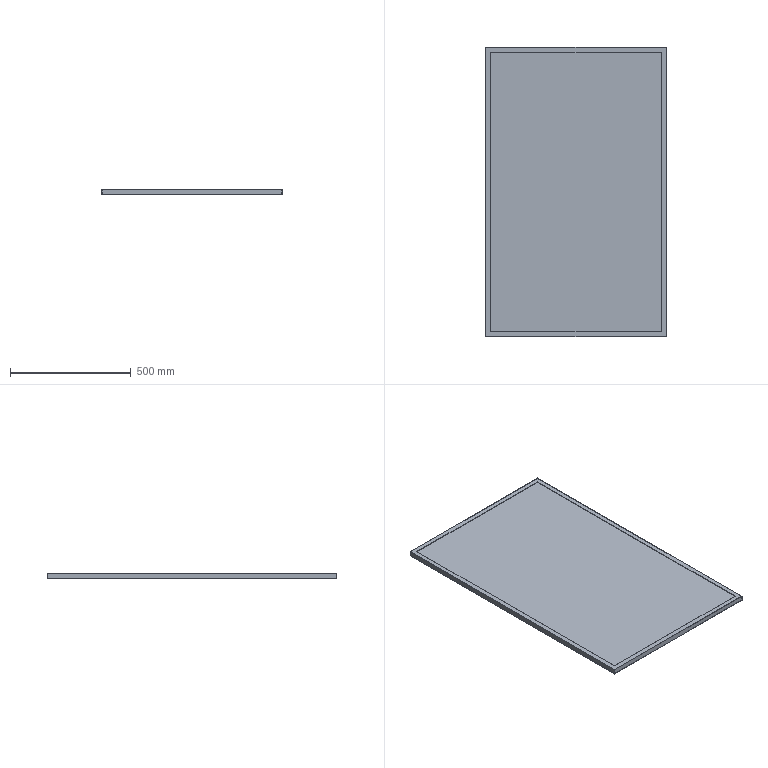Part | SolidWorks | features Extrusion 1, ICE 1, Shell 1 | 1 solid | 16 faces | box 745 x 1196 x 22 mm | volume 2073584 mm3 | plane 16
STEP:
#1=CARTESIAN_POINT('',(0.,1196.,22.));
#2=VERTEX_POINT('',#1);
#3=CARTESIAN_POINT('',(0.,0.,22.));
#4=VERTEX_POINT('',#3);
#5=CARTESIAN_POINT('',(0.,0.,22.));
#6=DIRECTION('',(0.,-1.,0.));
#7=VECTOR('',#6,1000.);
#8=LINE('',#5,#7);
#9=EDGE_CURVE('',#2,#4,#8,.T.);
#10=ORIENTED_EDGE('',*,*,#9,.T.);
#11=CARTESIAN_POINT('',(745.,0.,22.));
#12=VERTEX_POINT('',#11);
#13=CARTESIAN_POINT('',(0.,0.,22.));
#14=DIRECTION('',(1.,0.,0.));
#15=VECTOR('',#14,1000.);
#16=LINE('',#13,#15);
#17=EDGE_CURVE('',#4,#12,#16,.T.);
#18=ORIENTED_EDGE('',*,*,#17,.T.);
#19=CARTESIAN_POINT('',(745.,1196.,22.));
#20=VERTEX_POINT('',#19);
#21=CARTESIAN_POINT('',(745.,0.,22.));
#22=DIRECTION('',(0.,1.,0.));
#23=VECTOR('',#22,1000.);
#24=LINE('',#21,#23);
#25=EDGE_CURVE('',#12,#20,#24,.T.);
#26=ORIENTED_EDGE('',*,*,#25,.T.);
#27=CARTESIAN_POINT('',(0.,1196.,22.));
#28=DIRECTION('',(-1.,0.,0.));
#29=VECTOR('',#28,1000.);
#30=LINE('',#27,#29);
#31=EDGE_CURVE('',#20,#2,#30,.T.);
#32=ORIENTED_EDGE('',*,*,#31,.T.);
#33=EDGE_LOOP('',(#10,#18,#26,#32));
#34=FACE_OUTER_BOUND('',#33,.T.);
#35=CARTESIAN_POINT('',(725.,1176.,22.));
#36=VERTEX_POINT('',#35);
#37=CARTESIAN_POINT('',(20.,1176.,22.));
#38=VERTEX_POINT('',#37);
#39=CARTESIAN_POINT('',(725.,1176.,22.));
#40=DIRECTION('',(-1.,0.,0.));
#41=VECTOR('',#40,1000.);
#42=LINE('',#39,#41);
#43=EDGE_CURVE('',#36,#38,#42,.T.);
#44=ORIENTED_EDGE('',*,*,#43,.F.);
#45=CARTESIAN_POINT('',(725.,20.,22.));
#46=VERTEX_POINT('',#45);
#47=CARTESIAN_POINT('',(725.,20.,22.));
#48=DIRECTION('',(0.,1.,0.));
#49=VECTOR('',#48,1000.);
#50=LINE('',#47,#49);
#51=EDGE_CURVE('',#46,#36,#50,.T.);
#52=ORIENTED_EDGE('',*,*,#51,.F.);
#53=CARTESIAN_POINT('',(20.,20.,22.));
#54=VERTEX_POINT('',#53);
#55=CARTESIAN_POINT('',(20.,20.,22.));
#56=DIRECTION('',(1.,0.,0.));
#57=VECTOR('',#56,1000.);
#58=LINE('',#55,#57);
#59=EDGE_CURVE('',#54,#46,#58,.T.);
#60=ORIENTED_EDGE('',*,*,#59,.F.);
#61=CARTESIAN_POINT('',(20.,1176.,22.));
#62=DIRECTION('',(0.,-1.,0.));
#63=VECTOR('',#62,1000.);
#64=LINE('',#61,#63);
#65=EDGE_CURVE('',#38,#54,#64,.T.);
#66=ORIENTED_EDGE('',*,*,#65,.F.);
#67=EDGE_LOOP('',(#44,#52,#60,#66));
#68=FACE_BOUND('',#67,.T.);
#69=CARTESIAN_POINT('',(0.,1196.,22.));
#70=DIRECTION('',(0.,0.,-1.));
#71=DIRECTION('',(-1.,0.,0.));
#72=AXIS2_PLACEMENT_3D('',#69,#70,#71);
#73=PLANE('',#72);
#74=ADVANCED_FACE('',(#34,#68),#73,.F.);
#75=CARTESIAN_POINT('',(0.,1196.,0.));
#76=VERTEX_POINT('',#75);
#77=CARTESIAN_POINT('',(0.,1196.,22.));
#78=DIRECTION('',(0.,0.,-1.));
#79=VECTOR('',#78,1000.);
#80=LINE('',#77,#79);
#81=EDGE_CURVE('',#2,#76,#80,.T.);
#82=ORIENTED_EDGE('',*,*,#81,.T.);
#83=CARTESIAN_POINT('',(0.,0.,0.));
#84=VERTEX_POINT('',#83);
#85=CARTESIAN_POINT('',(0.,0.,0.));
#86=DIRECTION('',(0.,-1.,0.));
#87=VECTOR('',#86,1000.);
#88=LINE('',#85,#87);
#89=EDGE_CURVE('',#76,#84,#88,.T.);
#90=ORIENTED_EDGE('',*,*,#89,.T.);
#91=CARTESIAN_POINT('',(0.,0.,22.));
#92=DIRECTION('',(0.,0.,-1.));
#93=VECTOR('',#92,1000.);
#94=LINE('',#91,#93);
#95=EDGE_CURVE('',#4,#84,#94,.T.);
#96=ORIENTED_EDGE('',*,*,#95,.F.);
#97=ORIENTED_EDGE('',*,*,#9,.F.);
#98=EDGE_LOOP('',(#82,#90,#96,#97));
#99=FACE_OUTER_BOUND('',#98,.T.);
#100=CARTESIAN_POINT('',(0.,0.,22.));
#101=DIRECTION('',(1.,0.,0.));
#102=DIRECTION('',(0.,0.,-1.));
#103=AXIS2_PLACEMENT_3D('',#100,#101,#102);
#104=PLANE('',#103);
#105=ADVANCED_FACE('',(#99),#104,.F.);
#106=ORIENTED_EDGE('',*,*,#95,.T.);
#107=CARTESIAN_POINT('',(745.,0.,0.));
#108=VERTEX_POINT('',#107);
#109=CARTESIAN_POINT('',(0.,0.,0.));
#110=DIRECTION('',(1.,0.,0.));
#111=VECTOR('',#110,1000.);
#112=LINE('',#109,#111);
#113=EDGE_CURVE('',#84,#108,#112,.T.);
#114=ORIENTED_EDGE('',*,*,#113,.T.);
#115=CARTESIAN_POINT('',(745.,0.,22.));
#116=DIRECTION('',(0.,0.,-1.));
#117=VECTOR('',#116,1000.);
#118=LINE('',#115,#117);
#119=EDGE_CURVE('',#12,#108,#118,.T.);
#120=ORIENTED_EDGE('',*,*,#119,.F.);
#121=ORIENTED_EDGE('',*,*,#17,.F.);
#122=EDGE_LOOP('',(#106,#114,#120,#121));
#123=FACE_OUTER_BOUND('',#122,.T.);
#124=CARTESIAN_POINT('',(0.,0.,22.));
#125=DIRECTION('',(0.,1.,0.));
#126=DIRECTION('',(0.,0.,1.));
#127=AXIS2_PLACEMENT_3D('',#124,#125,#126);
#128=PLANE('',#127);
#129=ADVANCED_FACE('',(#123),#128,.F.);
#130=ORIENTED_EDGE('',*,*,#119,.T.);
#131=CARTESIAN_POINT('',(745.,1196.,0.));
#132=VERTEX_POINT('',#131);
#133=CARTESIAN_POINT('',(745.,0.,0.));
#134=DIRECTION('',(0.,1.,0.));
#135=VECTOR('',#134,1000.);
#136=LINE('',#133,#135);
#137=EDGE_CURVE('',#108,#132,#136,.T.);
#138=ORIENTED_EDGE('',*,*,#137,.T.);
#139=CARTESIAN_POINT('',(745.,1196.,22.));
#140=DIRECTION('',(0.,0.,-1.));
#141=VECTOR('',#140,1000.);
#142=LINE('',#139,#141);
#143=EDGE_CURVE('',#20,#132,#142,.T.);
#144=ORIENTED_EDGE('',*,*,#143,.F.);
#145=ORIENTED_EDGE('',*,*,#25,.F.);
#146=EDGE_LOOP('',(#130,#138,#144,#145));
#147=FACE_OUTER_BOUND('',#146,.T.);
#148=CARTESIAN_POINT('',(745.,0.,22.));
#149=DIRECTION('',(-1.,0.,0.));
#150=DIRECTION('',(0.,0.,1.));
#151=AXIS2_PLACEMENT_3D('',#148,#149,#150);
#152=PLANE('',#151);
#153=ADVANCED_FACE('',(#147),#152,.F.);
#154=ORIENTED_EDGE('',*,*,#143,.T.);
#155=CARTESIAN_POINT('',(0.,1196.,0.));
#156=DIRECTION('',(-1.,0.,0.));
#157=VECTOR('',#156,1000.);
#158=LINE('',#155,#157);
#159=EDGE_CURVE('',#132,#76,#158,.T.);
#160=ORIENTED_EDGE('',*,*,#159,.T.);
#161=ORIENTED_EDGE('',*,*,#81,.F.);
#162=ORIENTED_EDGE('',*,*,#31,.F.);
#163=EDGE_LOOP('',(#154,#160,#161,#162));
#164=FACE_OUTER_BOUND('',#163,.T.);
#165=CARTESIAN_POINT('',(0.,1196.,22.));
#166=DIRECTION('',(0.,-1.,0.));
#167=DIRECTION('',(0.,0.,-1.));
#168=AXIS2_PLACEMENT_3D('',#165,#166,#167);
#169=PLANE('',#168);
#170=ADVANCED_FACE('',(#164),#169,.F.);
#171=ORIENTED_EDGE('',*,*,#89,.F.);
#172=ORIENTED_EDGE('',*,*,#159,.F.);
#173=ORIENTED_EDGE('',*,*,#137,.F.);
#174=ORIENTED_EDGE('',*,*,#113,.F.);
#175=EDGE_LOOP('',(#171,#172,#173,#174));
#176=FACE_OUTER_BOUND('',#175,.T.);
#177=CARTESIAN_POINT('',(0.,1196.,0.));
#178=DIRECTION('',(0.,0.,-1.));
#179=DIRECTION('',(-1.,0.,0.));
#180=AXIS2_PLACEMENT_3D('',#177,#178,#179);
#181=PLANE('',#180);
#182=ADVANCED_FACE('',(#176),#181,.T.);
#183=CARTESIAN_POINT('',(2.,1194.,20.));
#184=VERTEX_POINT('',#183);
#185=CARTESIAN_POINT('',(2.,2.,20.));
#186=VERTEX_POINT('',#185);
#187=CARTESIAN_POINT('',(2.,0.,20.));
#188=DIRECTION('',(0.,-1.,0.));
#189=VECTOR('',#188,1000.);
#190=LINE('',#187,#189);
#191=EDGE_CURVE('',#184,#186,#190,.T.);
#192=ORIENTED_EDGE('',*,*,#191,.F.);
#193=CARTESIAN_POINT('',(743.,1194.,20.));
#194=VERTEX_POINT('',#193);
#195=CARTESIAN_POINT('',(0.,1194.,20.));
#196=DIRECTION('',(-1.,0.,0.));
#197=VECTOR('',#196,1000.);
#198=LINE('',#195,#197);
#199=EDGE_CURVE('',#194,#184,#198,.T.);
#200=ORIENTED_EDGE('',*,*,#199,.F.);
#201=CARTESIAN_POINT('',(743.,2.,20.));
#202=VERTEX_POINT('',#201);
#203=CARTESIAN_POINT('',(743.,0.,20.));
#204=DIRECTION('',(0.,1.,0.));
#205=VECTOR('',#204,1000.);
#206=LINE('',#203,#205);
#207=EDGE_CURVE('',#202,#194,#206,.T.);
#208=ORIENTED_EDGE('',*,*,#207,.F.);
#209=CARTESIAN_POINT('',(0.,2.,20.));
#210=DIRECTION('',(1.,0.,0.));
#211=VECTOR('',#210,1000.);
#212=LINE('',#209,#211);
#213=EDGE_CURVE('',#186,#202,#212,.T.);
#214=ORIENTED_EDGE('',*,*,#213,.F.);
#215=EDGE_LOOP('',(#192,#200,#208,#214));
#216=FACE_OUTER_BOUND('',#215,.T.);
#217=CARTESIAN_POINT('',(725.,20.,20.));
#218=VERTEX_POINT('',#217);
#219=CARTESIAN_POINT('',(725.,1176.,20.));
#220=VERTEX_POINT('',#219);
#221=CARTESIAN_POINT('',(725.,20.,20.));
#222=DIRECTION('',(0.,1.,0.));
#223=VECTOR('',#222,1000.);
#224=LINE('',#221,#223);
#225=EDGE_CURVE('',#218,#220,#224,.T.);
#226=ORIENTED_EDGE('',*,*,#225,.T.);
#227=CARTESIAN_POINT('',(20.,1176.,20.));
#228=VERTEX_POINT('',#227);
#229=CARTESIAN_POINT('',(725.,1176.,20.));
#230=DIRECTION('',(-1.,0.,0.));
#231=VECTOR('',#230,1000.);
#232=LINE('',#229,#231);
#233=EDGE_CURVE('',#220,#228,#232,.T.);
#234=ORIENTED_EDGE('',*,*,#233,.T.);
#235=CARTESIAN_POINT('',(20.,20.,20.));
#236=VERTEX_POINT('',#235);
#237=CARTESIAN_POINT('',(20.,1176.,20.));
#238=DIRECTION('',(0.,-1.,0.));
#239=VECTOR('',#238,1000.);
#240=LINE('',#237,#239);
#241=EDGE_CURVE('',#228,#236,#240,.T.);
#242=ORIENTED_EDGE('',*,*,#241,.T.);
#243=CARTESIAN_POINT('',(20.,20.,20.));
#244=DIRECTION('',(1.,0.,0.));
#245=VECTOR('',#244,1000.);
#246=LINE('',#243,#245);
#247=EDGE_CURVE('',#236,#218,#246,.T.);
#248=ORIENTED_EDGE('',*,*,#247,.T.);
#249=EDGE_LOOP('',(#226,#234,#242,#248));
#250=FACE_BOUND('',#249,.T.);
#251=CARTESIAN_POINT('',(0.,1196.,20.));
#252=DIRECTION('',(0.,0.,1.));
#253=DIRECTION('',(1.,0.,0.));
#254=AXIS2_PLACEMENT_3D('',#251,#252,#253);
#255=PLANE('',#254);
#256=ADVANCED_FACE('',(#216,#250),#255,.F.);
#257=ORIENTED_EDGE('',*,*,#43,.T.);
#258=CARTESIAN_POINT('',(20.,1176.,20.));
#259=DIRECTION('',(0.,0.,1.));
#260=VECTOR('',#259,1000.);
#261=LINE('',#258,#260);
#262=EDGE_CURVE('',#228,#38,#261,.T.);
#263=ORIENTED_EDGE('',*,*,#262,.F.);
#264=ORIENTED_EDGE('',*,*,#233,.F.);
#265=CARTESIAN_POINT('',(725.,1176.,20.));
#266=DIRECTION('',(0.,0.,1.));
#267=VECTOR('',#266,1000.);
#268=LINE('',#265,#267);
#269=EDGE_CURVE('',#220,#36,#268,.T.);
#270=ORIENTED_EDGE('',*,*,#269,.T.);
#271=EDGE_LOOP('',(#257,#263,#264,#270));
#272=FACE_OUTER_BOUND('',#271,.T.);
#273=CARTESIAN_POINT('',(725.,1176.,20.));
#274=DIRECTION('',(0.,1.,0.));
#275=DIRECTION('',(0.,0.,1.));
#276=AXIS2_PLACEMENT_3D('',#273,#274,#275);
#277=PLANE('',#276);
#278=ADVANCED_FACE('',(#272),#277,.F.);
#279=ORIENTED_EDGE('',*,*,#51,.T.);
#280=ORIENTED_EDGE('',*,*,#269,.F.);
#281=ORIENTED_EDGE('',*,*,#225,.F.);
#282=CARTESIAN_POINT('',(725.,20.,20.));
#283=DIRECTION('',(0.,0.,1.));
#284=VECTOR('',#283,1000.);
#285=LINE('',#282,#284);
#286=EDGE_CURVE('',#218,#46,#285,.T.);
#287=ORIENTED_EDGE('',*,*,#286,.T.);
#288=EDGE_LOOP('',(#279,#280,#281,#287));
#289=FACE_OUTER_BOUND('',#288,.T.);
#290=CARTESIAN_POINT('',(725.,20.,20.));
#291=DIRECTION('',(1.,0.,0.));
#292=DIRECTION('',(0.,0.,-1.));
#293=AXIS2_PLACEMENT_3D('',#290,#291,#292);
#294=PLANE('',#293);
#295=ADVANCED_FACE('',(#289),#294,.F.);
#296=ORIENTED_EDGE('',*,*,#59,.T.);
#297=ORIENTED_EDGE('',*,*,#286,.F.);
#298=ORIENTED_EDGE('',*,*,#247,.F.);
#299=CARTESIAN_POINT('',(20.,20.,20.));
#300=DIRECTION('',(0.,0.,1.));
#301=VECTOR('',#300,1000.);
#302=LINE('',#299,#301);
#303=EDGE_CURVE('',#236,#54,#302,.T.);
#304=ORIENTED_EDGE('',*,*,#303,.T.);
#305=EDGE_LOOP('',(#296,#297,#298,#304));
#306=FACE_OUTER_BOUND('',#305,.T.);
#307=CARTESIAN_POINT('',(20.,20.,20.));
#308=DIRECTION('',(0.,-1.,0.));
#309=DIRECTION('',(0.,0.,-1.));
#310=AXIS2_PLACEMENT_3D('',#307,#308,#309);
#311=PLANE('',#310);
#312=ADVANCED_FACE('',(#306),#311,.F.);
#313=ORIENTED_EDGE('',*,*,#65,.T.);
#314=ORIENTED_EDGE('',*,*,#303,.F.);
#315=ORIENTED_EDGE('',*,*,#241,.F.);
#316=ORIENTED_EDGE('',*,*,#262,.T.);
#317=EDGE_LOOP('',(#313,#314,#315,#316));
#318=FACE_OUTER_BOUND('',#317,.T.);
#319=CARTESIAN_POINT('',(20.,1176.,20.));
#320=DIRECTION('',(-1.,0.,0.));
#321=DIRECTION('',(0.,0.,1.));
#322=AXIS2_PLACEMENT_3D('',#319,#320,#321);
#323=PLANE('',#322);
#324=ADVANCED_FACE('',(#318),#323,.F.);
#325=CARTESIAN_POINT('',(2.,1194.,2.));
#326=VERTEX_POINT('',#325);
#327=CARTESIAN_POINT('',(2.,2.,2.));
#328=VERTEX_POINT('',#327);
#329=CARTESIAN_POINT('',(2.,1196.,2.));
#330=DIRECTION('',(0.,-1.,0.));
#331=VECTOR('',#330,1000.);
#332=LINE('',#329,#331);
#333=EDGE_CURVE('',#326,#328,#332,.T.);
#334=ORIENTED_EDGE('',*,*,#333,.T.);
#335=CARTESIAN_POINT('',(743.,2.,2.));
#336=VERTEX_POINT('',#335);
#337=CARTESIAN_POINT('',(0.,2.,2.));
#338=DIRECTION('',(1.,0.,0.));
#339=VECTOR('',#338,1000.);
#340=LINE('',#337,#339);
#341=EDGE_CURVE('',#328,#336,#340,.T.);
#342=ORIENTED_EDGE('',*,*,#341,.T.);
#343=CARTESIAN_POINT('',(743.,1194.,2.));
#344=VERTEX_POINT('',#343);
#345=CARTESIAN_POINT('',(743.,1196.,2.));
#346=DIRECTION('',(0.,1.,0.));
#347=VECTOR('',#346,1000.);
#348=LINE('',#345,#347);
#349=EDGE_CURVE('',#336,#344,#348,.T.);
#350=ORIENTED_EDGE('',*,*,#349,.T.);
#351=CARTESIAN_POINT('',(0.,1194.,2.));
#352=DIRECTION('',(-1.,0.,0.));
#353=VECTOR('',#352,1000.);
#354=LINE('',#351,#353);
#355=EDGE_CURVE('',#344,#326,#354,.T.);
#356=ORIENTED_EDGE('',*,*,#355,.T.);
#357=EDGE_LOOP('',(#334,#342,#350,#356));
#358=FACE_OUTER_BOUND('',#357,.T.);
#359=CARTESIAN_POINT('',(0.,1196.,2.));
#360=DIRECTION('',(0.,0.,-1.));
#361=DIRECTION('',(-1.,0.,0.));
#362=AXIS2_PLACEMENT_3D('',#359,#360,#361);
#363=PLANE('',#362);
#364=ADVANCED_FACE('',(#358),#363,.F.);
#365=CARTESIAN_POINT('',(743.,1194.,22.));
#366=DIRECTION('',(0.,0.,-1.));
#367=VECTOR('',#366,1000.);
#368=LINE('',#365,#367);
#369=EDGE_CURVE('',#194,#344,#368,.T.);
#370=ORIENTED_EDGE('',*,*,#369,.F.);
#371=ORIENTED_EDGE('',*,*,#199,.T.);
#372=CARTESIAN_POINT('',(2.,1194.,22.));
#373=DIRECTION('',(0.,0.,-1.));
#374=VECTOR('',#373,1000.);
#375=LINE('',#372,#374);
#376=EDGE_CURVE('',#184,#326,#375,.T.);
#377=ORIENTED_EDGE('',*,*,#376,.T.);
#378=ORIENTED_EDGE('',*,*,#355,.F.);
#379=EDGE_LOOP('',(#370,#371,#377,#378));
#380=FACE_OUTER_BOUND('',#379,.T.);
#381=CARTESIAN_POINT('',(0.,1194.,22.));
#382=DIRECTION('',(0.,-1.,0.));
#383=DIRECTION('',(0.,0.,-1.));
#384=AXIS2_PLACEMENT_3D('',#381,#382,#383);
#385=PLANE('',#384);
#386=ADVANCED_FACE('',(#380),#385,.T.);
#387=CARTESIAN_POINT('',(743.,2.,22.));
#388=DIRECTION('',(0.,0.,-1.));
#389=VECTOR('',#388,1000.);
#390=LINE('',#387,#389);
#391=EDGE_CURVE('',#202,#336,#390,.T.);
#392=ORIENTED_EDGE('',*,*,#391,.F.);
#393=ORIENTED_EDGE('',*,*,#207,.T.);
#394=ORIENTED_EDGE('',*,*,#369,.T.);
#395=ORIENTED_EDGE('',*,*,#349,.F.);
#396=EDGE_LOOP('',(#392,#393,#394,#395));
#397=FACE_OUTER_BOUND('',#396,.T.);
#398=CARTESIAN_POINT('',(743.,0.,22.));
#399=DIRECTION('',(-1.,0.,0.));
#400=DIRECTION('',(0.,0.,1.));
#401=AXIS2_PLACEMENT_3D('',#398,#399,#400);
#402=PLANE('',#401);
#403=ADVANCED_FACE('',(#397),#402,.T.);
#404=CARTESIAN_POINT('',(2.,2.,22.));
#405=DIRECTION('',(0.,0.,-1.));
#406=VECTOR('',#405,1000.);
#407=LINE('',#404,#406);
#408=EDGE_CURVE('',#186,#328,#407,.T.);
#409=ORIENTED_EDGE('',*,*,#408,.F.);
#410=ORIENTED_EDGE('',*,*,#213,.T.);
#411=ORIENTED_EDGE('',*,*,#391,.T.);
#412=ORIENTED_EDGE('',*,*,#341,.F.);
#413=EDGE_LOOP('',(#409,#410,#411,#412));
#414=FACE_OUTER_BOUND('',#413,.T.);
#415=CARTESIAN_POINT('',(0.,2.,22.));
#416=DIRECTION('',(0.,1.,0.));
#417=DIRECTION('',(0.,0.,1.));
#418=AXIS2_PLACEMENT_3D('',#415,#416,#417);
#419=PLANE('',#418);
#420=ADVANCED_FACE('',(#414),#419,.T.);
#421=ORIENTED_EDGE('',*,*,#376,.F.);
#422=ORIENTED_EDGE('',*,*,#191,.T.);
#423=ORIENTED_EDGE('',*,*,#408,.T.);
#424=ORIENTED_EDGE('',*,*,#333,.F.);
#425=EDGE_LOOP('',(#421,#422,#423,#424));
#426=FACE_OUTER_BOUND('',#425,.T.);
#427=CARTESIAN_POINT('',(2.,0.,22.));
#428=DIRECTION('',(1.,0.,0.));
#429=DIRECTION('',(0.,0.,-1.));
#430=AXIS2_PLACEMENT_3D('',#427,#428,#429);
#431=PLANE('',#430);
#432=ADVANCED_FACE('',(#426),#431,.T.);
#433=CLOSED_SHELL('',(#74,#105,#129,#153,#170,#182,#256,#278,#295,#312,#324,#364,#386,#403,#420,#432));
#434=MANIFOLD_SOLID_BREP('',#433);
#435=CARTESIAN_POINT('',(0.,0.,0.));
#436=DIRECTION('',(0.,0.,1.));
#437=DIRECTION('',(1.,0.,0.));
#438=AXIS2_PLACEMENT_3D('',#435,#436,#437);
#439=(LENGTH_UNIT()NAMED_UNIT(*)SI_UNIT(.MILLI.,.METRE.));
#440=UNCERTAINTY_MEASURE_WITH_UNIT(LENGTH_MEASURE(0.00001),#439,'','');
#441=(NAMED_UNIT(*)PLANE_ANGLE_UNIT()SI_UNIT($,.RADIAN.));
#442=(NAMED_UNIT(*)SI_UNIT($,.STERADIAN.)SOLID_ANGLE_UNIT());
#443=(GEOMETRIC_REPRESENTATION_CONTEXT(3)GLOBAL_UNCERTAINTY_ASSIGNED_CONTEXT((#440))GLOBAL_UNIT_ASSIGNED_CONTEXT((#439,#441,#442))REPRESENTATION_CONTEXT('',''));
#444=ADVANCED_BREP_SHAPE_REPRESENTATION('',(#434,#438),#443);